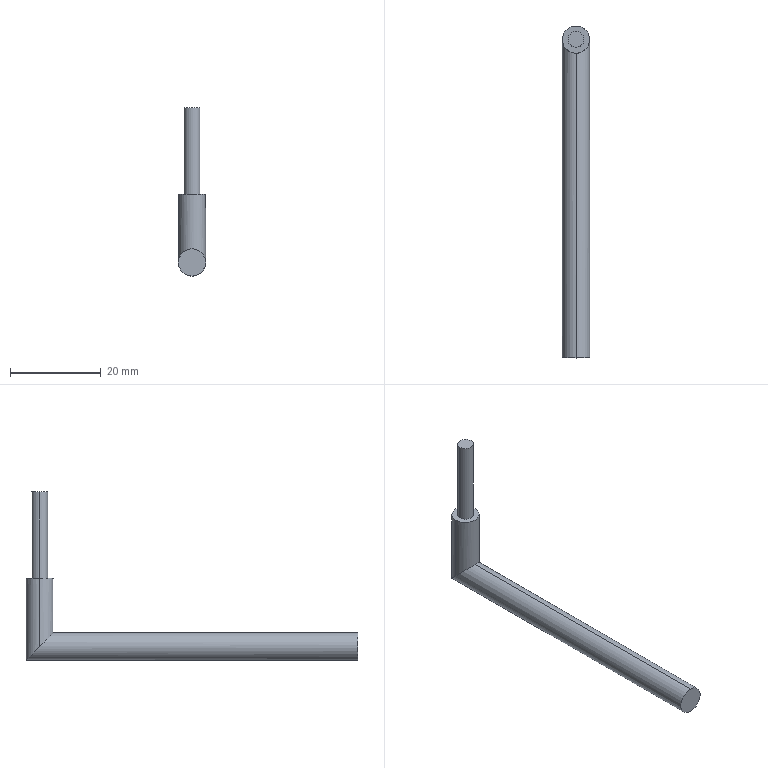Part | SolidWorks | features ICE 4, Extrusion 1 | 1 solid | 9 faces | box 6 x 73 x 37 mm | volume 2586 mm3 | cylinder 6 | plane 3 | commonest cylinder face diameters 6 x4 3.5 x2
STEP:
#1=CARTESIAN_POINT('',(1.75,70.,34.));
#2=VERTEX_POINT('',#1);
#3=CARTESIAN_POINT('',(-1.75,70.,34.));
#4=VERTEX_POINT('',#3);
#5=CARTESIAN_POINT('',(0.,70.,34.));
#6=DIRECTION('',(0.,0.,1.));
#7=DIRECTION('',(1.,0.,0.));
#8=AXIS2_PLACEMENT_3D('',#5,#6,#7);
#9=CIRCLE('',#8,1.75);
#10=EDGE_CURVE('',#2,#4,#9,.T.);
#11=ORIENTED_EDGE('',*,*,#10,.F.);
#12=CARTESIAN_POINT('',(1.75,70.,15.));
#13=VERTEX_POINT('',#12);
#14=CARTESIAN_POINT('',(1.75,70.,34.));
#15=DIRECTION('',(0.,0.,-1.));
#16=VECTOR('',#15,1000.);
#17=LINE('',#14,#16);
#18=EDGE_CURVE('',#2,#13,#17,.T.);
#19=ORIENTED_EDGE('',*,*,#18,.T.);
#20=CARTESIAN_POINT('',(-1.75,70.,15.));
#21=VERTEX_POINT('',#20);
#22=CARTESIAN_POINT('',(0.,70.,15.));
#23=DIRECTION('',(0.,0.,1.));
#24=DIRECTION('',(1.,0.,0.));
#25=AXIS2_PLACEMENT_3D('',#22,#23,#24);
#26=CIRCLE('',#25,1.75);
#27=EDGE_CURVE('',#13,#21,#26,.T.);
#28=ORIENTED_EDGE('',*,*,#27,.T.);
#29=CARTESIAN_POINT('',(-1.75,70.,34.));
#30=DIRECTION('',(0.,0.,-1.));
#31=VECTOR('',#30,1000.);
#32=LINE('',#29,#31);
#33=EDGE_CURVE('',#4,#21,#32,.T.);
#34=ORIENTED_EDGE('',*,*,#33,.F.);
#35=EDGE_LOOP('',(#11,#19,#28,#34));
#36=FACE_OUTER_BOUND('',#35,.T.);
#37=CARTESIAN_POINT('',(0.,70.,34.));
#38=DIRECTION('',(0.,0.,-1.));
#39=DIRECTION('',(-1.,0.,0.));
#40=AXIS2_PLACEMENT_3D('',#37,#38,#39);
#41=CYLINDRICAL_SURFACE('',#40,1.75);
#42=ADVANCED_FACE('',(#36),#41,.T.);
#43=CARTESIAN_POINT('',(3.,70.,15.));
#44=VERTEX_POINT('',#43);
#45=CARTESIAN_POINT('',(-3.,70.,15.));
#46=VERTEX_POINT('',#45);
#47=CARTESIAN_POINT('',(0.,70.,15.));
#48=DIRECTION('',(0.,0.,1.));
#49=DIRECTION('',(1.,0.,0.));
#50=AXIS2_PLACEMENT_3D('',#47,#48,#49);
#51=CIRCLE('',#50,3.);
#52=EDGE_CURVE('',#44,#46,#51,.T.);
#53=ORIENTED_EDGE('',*,*,#52,.F.);
#54=CARTESIAN_POINT('',(3.,70.,0.));
#55=VERTEX_POINT('',#54);
#56=CARTESIAN_POINT('',(3.,70.,15.));
#57=DIRECTION('',(0.,0.,-1.));
#58=VECTOR('',#57,1000.);
#59=LINE('',#56,#58);
#60=EDGE_CURVE('',#44,#55,#59,.T.);
#61=ORIENTED_EDGE('',*,*,#60,.T.);
#62=CARTESIAN_POINT('',(0.,73.,-3.));
#63=VERTEX_POINT('',#62);
#64=CARTESIAN_POINT('',(3.,70.,0.));
#65=CARTESIAN_POINT('',(3.,71.757,-1.757));
#66=CARTESIAN_POINT('',(1.757,73.,-3.));
#67=CARTESIAN_POINT('',(0.,73.,-3.));
#68=(BOUNDED_CURVE()B_SPLINE_CURVE(3,(#64,#65,#66,#67),.UNSPECIFIED.,.F.,.F.)B_SPLINE_CURVE_WITH_KNOTS((4,4),(1.571,3.142),.UNSPECIFIED.)CURVE()GEOMETRIC_REPRESENTATION_ITEM()RATIONAL_B_SPLINE_CURVE((1.,0.8047,0.8047,1.))REPRESENTATION_ITEM(''));
#69=EDGE_CURVE('',#55,#63,#68,.T.);
#70=ORIENTED_EDGE('',*,*,#69,.T.);
#71=CARTESIAN_POINT('',(-3.,70.,0.));
#72=VERTEX_POINT('',#71);
#73=CARTESIAN_POINT('',(0.,73.,-3.));
#74=CARTESIAN_POINT('',(-1.757,73.,-3.));
#75=CARTESIAN_POINT('',(-3.,71.757,-1.757));
#76=CARTESIAN_POINT('',(-3.,70.,0.));
#77=(BOUNDED_CURVE()B_SPLINE_CURVE(3,(#73,#74,#75,#76),.UNSPECIFIED.,.F.,.T.)B_SPLINE_CURVE_WITH_KNOTS((4,4),(3.142,4.712),.UNSPECIFIED.)CURVE()GEOMETRIC_REPRESENTATION_ITEM()RATIONAL_B_SPLINE_CURVE((1.,0.8047,0.8047,1.))REPRESENTATION_ITEM(''));
#78=EDGE_CURVE('',#63,#72,#77,.T.);
#79=ORIENTED_EDGE('',*,*,#78,.T.);
#80=CARTESIAN_POINT('',(-3.,70.,15.));
#81=DIRECTION('',(0.,0.,-1.));
#82=VECTOR('',#81,1000.);
#83=LINE('',#80,#82);
#84=EDGE_CURVE('',#46,#72,#83,.T.);
#85=ORIENTED_EDGE('',*,*,#84,.F.);
#86=EDGE_LOOP('',(#53,#61,#70,#79,#85));
#87=FACE_OUTER_BOUND('',#86,.T.);
#88=CARTESIAN_POINT('',(0.,70.,15.));
#89=DIRECTION('',(0.,0.,-1.));
#90=DIRECTION('',(-1.,0.,0.));
#91=AXIS2_PLACEMENT_3D('',#88,#89,#90);
#92=CYLINDRICAL_SURFACE('',#91,3.);
#93=ADVANCED_FACE('',(#87),#92,.T.);
#94=CARTESIAN_POINT('',(0.,67.,3.));
#95=VERTEX_POINT('',#94);
#96=CARTESIAN_POINT('',(0.,67.,3.));
#97=CARTESIAN_POINT('',(1.757,67.,3.));
#98=CARTESIAN_POINT('',(3.,68.243,1.757));
#99=CARTESIAN_POINT('',(3.,70.,0.));
#100=(BOUNDED_CURVE()B_SPLINE_CURVE(3,(#96,#97,#98,#99),.UNSPECIFIED.,.F.,.T.)B_SPLINE_CURVE_WITH_KNOTS((4,4),(0.,1.571),.UNSPECIFIED.)CURVE()GEOMETRIC_REPRESENTATION_ITEM()RATIONAL_B_SPLINE_CURVE((1.,0.8047,0.8047,1.))REPRESENTATION_ITEM(''));
#101=EDGE_CURVE('',#95,#55,#100,.T.);
#102=ORIENTED_EDGE('',*,*,#101,.F.);
#103=CARTESIAN_POINT('',(0.,0.,3.));
#104=VERTEX_POINT('',#103);
#105=CARTESIAN_POINT('',(0.,70.,3.));
#106=DIRECTION('',(0.,-1.,0.));
#107=VECTOR('',#106,1000.);
#108=LINE('',#105,#107);
#109=EDGE_CURVE('',#95,#104,#108,.T.);
#110=ORIENTED_EDGE('',*,*,#109,.T.);
#111=CARTESIAN_POINT('',(0.,0.,-3.));
#112=VERTEX_POINT('',#111);
#113=CARTESIAN_POINT('',(0.,0.,0.));
#114=DIRECTION('',(0.,1.,0.));
#115=DIRECTION('',(0.,0.,1.));
#116=AXIS2_PLACEMENT_3D('',#113,#114,#115);
#117=CIRCLE('',#116,3.);
#118=EDGE_CURVE('',#104,#112,#117,.T.);
#119=ORIENTED_EDGE('',*,*,#118,.T.);
#120=CARTESIAN_POINT('',(0.,70.,-3.));
#121=DIRECTION('',(0.,-1.,0.));
#122=VECTOR('',#121,1000.);
#123=LINE('',#120,#122);
#124=EDGE_CURVE('',#63,#112,#123,.T.);
#125=ORIENTED_EDGE('',*,*,#124,.F.);
#126=ORIENTED_EDGE('',*,*,#69,.F.);
#127=EDGE_LOOP('',(#102,#110,#119,#125,#126));
#128=FACE_OUTER_BOUND('',#127,.T.);
#129=CARTESIAN_POINT('',(0.,70.,0.));
#130=DIRECTION('',(0.,-1.,0.));
#131=DIRECTION('',(0.,0.,-1.));
#132=AXIS2_PLACEMENT_3D('',#129,#130,#131);
#133=CYLINDRICAL_SURFACE('',#132,3.);
#134=ADVANCED_FACE('',(#128),#133,.T.);
#135=CARTESIAN_POINT('',(0.,70.,15.));
#136=DIRECTION('',(0.,0.,1.));
#137=DIRECTION('',(1.,0.,0.));
#138=AXIS2_PLACEMENT_3D('',#135,#136,#137);
#139=CIRCLE('',#138,3.);
#140=EDGE_CURVE('',#46,#44,#139,.T.);
#141=ORIENTED_EDGE('',*,*,#140,.T.);
#142=ORIENTED_EDGE('',*,*,#52,.T.);
#143=EDGE_LOOP('',(#141,#142));
#144=FACE_OUTER_BOUND('',#143,.T.);
#145=CARTESIAN_POINT('',(0.,70.,15.));
#146=DIRECTION('',(0.,0.,1.));
#147=DIRECTION('',(1.,0.,0.));
#148=AXIS2_PLACEMENT_3D('',#145,#146,#147);
#149=CIRCLE('',#148,1.75);
#150=EDGE_CURVE('',#21,#13,#149,.T.);
#151=ORIENTED_EDGE('',*,*,#150,.F.);
#152=ORIENTED_EDGE('',*,*,#27,.F.);
#153=EDGE_LOOP('',(#151,#152));
#154=FACE_BOUND('',#153,.T.);
#155=CARTESIAN_POINT('',(0.,70.,15.));
#156=DIRECTION('',(0.,0.,1.));
#157=DIRECTION('',(1.,0.,0.));
#158=AXIS2_PLACEMENT_3D('',#155,#156,#157);
#159=PLANE('',#158);
#160=ADVANCED_FACE('',(#144,#154),#159,.T.);
#161=ORIENTED_EDGE('',*,*,#109,.F.);
#162=CARTESIAN_POINT('',(-3.,70.,0.));
#163=CARTESIAN_POINT('',(-3.,68.243,1.757));
#164=CARTESIAN_POINT('',(-1.757,67.,3.));
#165=CARTESIAN_POINT('',(0.,67.,3.));
#166=(BOUNDED_CURVE()B_SPLINE_CURVE(3,(#162,#163,#164,#165),.UNSPECIFIED.,.F.,.F.)B_SPLINE_CURVE_WITH_KNOTS((4,4),(4.712,6.283),.UNSPECIFIED.)CURVE()GEOMETRIC_REPRESENTATION_ITEM()RATIONAL_B_SPLINE_CURVE((1.,0.8047,0.8047,1.))REPRESENTATION_ITEM(''));
#167=EDGE_CURVE('',#72,#95,#166,.T.);
#168=ORIENTED_EDGE('',*,*,#167,.F.);
#169=ORIENTED_EDGE('',*,*,#78,.F.);
#170=ORIENTED_EDGE('',*,*,#124,.T.);
#171=CARTESIAN_POINT('',(0.,0.,0.));
#172=DIRECTION('',(0.,1.,0.));
#173=DIRECTION('',(0.,0.,1.));
#174=AXIS2_PLACEMENT_3D('',#171,#172,#173);
#175=CIRCLE('',#174,3.);
#176=EDGE_CURVE('',#112,#104,#175,.T.);
#177=ORIENTED_EDGE('',*,*,#176,.T.);
#178=EDGE_LOOP('',(#161,#168,#169,#170,#177));
#179=FACE_OUTER_BOUND('',#178,.T.);
#180=CARTESIAN_POINT('',(0.,70.,0.));
#181=DIRECTION('',(0.,-1.,0.));
#182=DIRECTION('',(0.,0.,-1.));
#183=AXIS2_PLACEMENT_3D('',#180,#181,#182);
#184=CYLINDRICAL_SURFACE('',#183,3.);
#185=ADVANCED_FACE('',(#179),#184,.T.);
#186=ORIENTED_EDGE('',*,*,#176,.F.);
#187=ORIENTED_EDGE('',*,*,#118,.F.);
#188=EDGE_LOOP('',(#186,#187));
#189=FACE_OUTER_BOUND('',#188,.T.);
#190=CARTESIAN_POINT('',(0.,0.,0.));
#191=DIRECTION('',(0.,1.,0.));
#192=DIRECTION('',(0.,0.,1.));
#193=AXIS2_PLACEMENT_3D('',#190,#191,#192);
#194=PLANE('',#193);
#195=ADVANCED_FACE('',(#189),#194,.F.);
#196=ORIENTED_EDGE('',*,*,#60,.F.);
#197=ORIENTED_EDGE('',*,*,#140,.F.);
#198=ORIENTED_EDGE('',*,*,#84,.T.);
#199=ORIENTED_EDGE('',*,*,#167,.T.);
#200=ORIENTED_EDGE('',*,*,#101,.T.);
#201=EDGE_LOOP('',(#196,#197,#198,#199,#200));
#202=FACE_OUTER_BOUND('',#201,.T.);
#203=CARTESIAN_POINT('',(0.,70.,15.));
#204=DIRECTION('',(0.,0.,-1.));
#205=DIRECTION('',(-1.,0.,0.));
#206=AXIS2_PLACEMENT_3D('',#203,#204,#205);
#207=CYLINDRICAL_SURFACE('',#206,3.);
#208=ADVANCED_FACE('',(#202),#207,.T.);
#209=ORIENTED_EDGE('',*,*,#18,.F.);
#210=CARTESIAN_POINT('',(0.,70.,34.));
#211=DIRECTION('',(0.,0.,1.));
#212=DIRECTION('',(1.,0.,0.));
#213=AXIS2_PLACEMENT_3D('',#210,#211,#212);
#214=CIRCLE('',#213,1.75);
#215=EDGE_CURVE('',#4,#2,#214,.T.);
#216=ORIENTED_EDGE('',*,*,#215,.F.);
#217=ORIENTED_EDGE('',*,*,#33,.T.);
#218=ORIENTED_EDGE('',*,*,#150,.T.);
#219=EDGE_LOOP('',(#209,#216,#217,#218));
#220=FACE_OUTER_BOUND('',#219,.T.);
#221=CARTESIAN_POINT('',(0.,70.,34.));
#222=DIRECTION('',(0.,0.,-1.));
#223=DIRECTION('',(-1.,0.,0.));
#224=AXIS2_PLACEMENT_3D('',#221,#222,#223);
#225=CYLINDRICAL_SURFACE('',#224,1.75);
#226=ADVANCED_FACE('',(#220),#225,.T.);
#227=ORIENTED_EDGE('',*,*,#215,.T.);
#228=ORIENTED_EDGE('',*,*,#10,.T.);
#229=EDGE_LOOP('',(#227,#228));
#230=FACE_OUTER_BOUND('',#229,.T.);
#231=CARTESIAN_POINT('',(0.,70.,34.));
#232=DIRECTION('',(0.,0.,1.));
#233=DIRECTION('',(1.,0.,0.));
#234=AXIS2_PLACEMENT_3D('',#231,#232,#233);
#235=PLANE('',#234);
#236=ADVANCED_FACE('',(#230),#235,.T.);
#237=CLOSED_SHELL('',(#42,#93,#134,#160,#185,#195,#208,#226,#236));
#238=MANIFOLD_SOLID_BREP('',#237);
#239=CARTESIAN_POINT('',(0.,0.,0.));
#240=DIRECTION('',(0.,0.,1.));
#241=DIRECTION('',(1.,0.,0.));
#242=AXIS2_PLACEMENT_3D('',#239,#240,#241);
#243=(LENGTH_UNIT()NAMED_UNIT(*)SI_UNIT(.MILLI.,.METRE.));
#244=UNCERTAINTY_MEASURE_WITH_UNIT(LENGTH_MEASURE(0.00001),#243,'','');
#245=(NAMED_UNIT(*)PLANE_ANGLE_UNIT()SI_UNIT($,.RADIAN.));
#246=(NAMED_UNIT(*)SI_UNIT($,.STERADIAN.)SOLID_ANGLE_UNIT());
#247=(GEOMETRIC_REPRESENTATION_CONTEXT(3)GLOBAL_UNCERTAINTY_ASSIGNED_CONTEXT((#244))GLOBAL_UNIT_ASSIGNED_CONTEXT((#243,#245,#246))REPRESENTATION_CONTEXT('',''));
#248=ADVANCED_BREP_SHAPE_REPRESENTATION('',(#238,#242),#247);